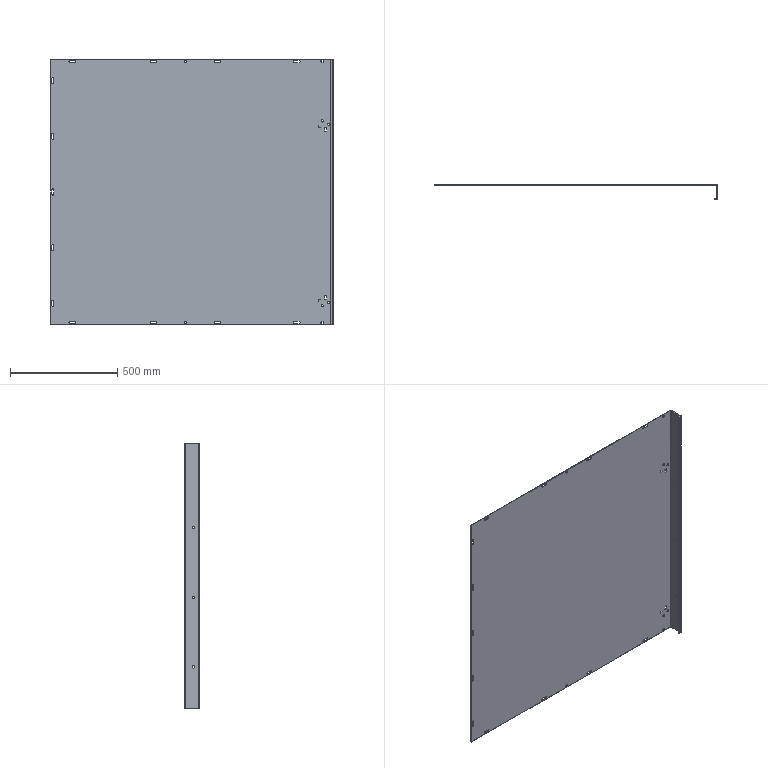Part | 1 solid | 127 faces | box 1320 x 70 x 1240 mm | volume 5184090 mm3 | plane 68 | cylinder 59 | commonest cylinder face diameters 10 x35 10.5 x14 8 x4 0.4 x2 4 x2 6.4 x2